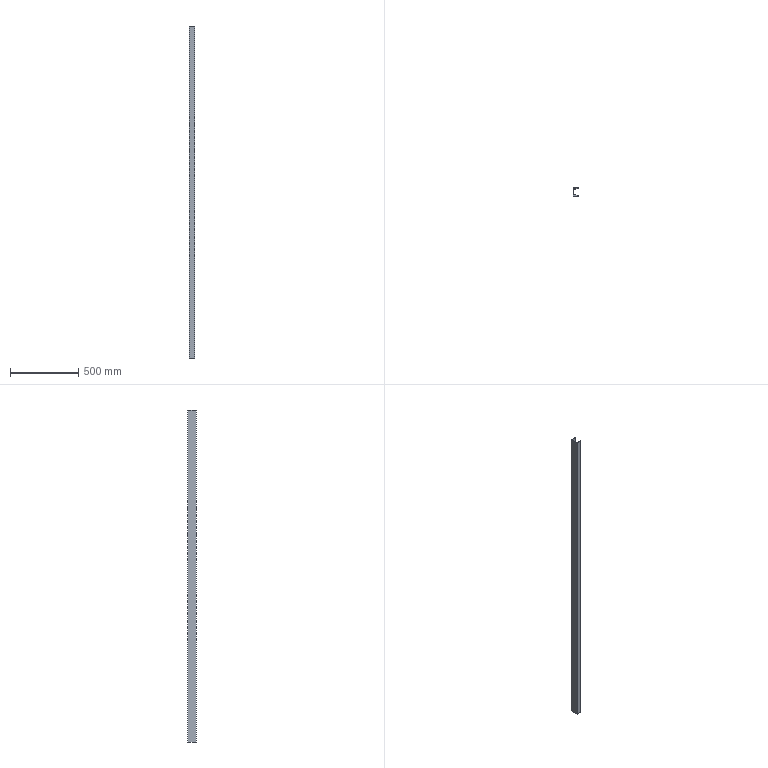Part | STEP file | 750038454 | 1 solid | 14 faces | box 40 x 63 x 2434 mm | volume 2055677 mm3 | plane 10 | cylinder 4 | commonest cylinder face diameters 7.6 x2 15 x2
STEP:
#1=CARTESIAN_POINT('',(0.,0.,2434.));
#2=VERTEX_POINT('',#1);
#3=CARTESIAN_POINT('',(0.,0.,0.));
#4=VERTEX_POINT('',#3);
#5=CARTESIAN_POINT('',(0.,0.,2434.));
#6=DIRECTION('',(0.,0.,-1.));
#7=VECTOR('',#6,1000.);
#8=LINE('',#5,#7);
#9=EDGE_CURVE('',#2,#4,#8,.T.);
#10=ORIENTED_EDGE('',*,*,#9,.F.);
#11=CARTESIAN_POINT('',(0.,63.,2434.));
#12=VERTEX_POINT('',#11);
#13=CARTESIAN_POINT('',(0.,63.,2434.));
#14=DIRECTION('',(0.,-1.,0.));
#15=VECTOR('',#14,1000.);
#16=LINE('',#13,#15);
#17=EDGE_CURVE('',#12,#2,#16,.T.);
#18=ORIENTED_EDGE('',*,*,#17,.F.);
#19=CARTESIAN_POINT('',(0.,63.,0.));
#20=VERTEX_POINT('',#19);
#21=CARTESIAN_POINT('',(0.,63.,2434.));
#22=DIRECTION('',(0.,0.,1.));
#23=VECTOR('',#22,1000.);
#24=LINE('',#21,#23);
#25=EDGE_CURVE('',#20,#12,#24,.T.);
#26=ORIENTED_EDGE('',*,*,#25,.F.);
#27=CARTESIAN_POINT('',(0.,63.,0.));
#28=DIRECTION('',(0.,1.,0.));
#29=VECTOR('',#28,1000.);
#30=LINE('',#27,#29);
#31=EDGE_CURVE('',#4,#20,#30,.T.);
#32=ORIENTED_EDGE('',*,*,#31,.F.);
#33=EDGE_LOOP('',(#10,#18,#26,#32));
#34=FACE_OUTER_BOUND('',#33,.T.);
#35=CARTESIAN_POINT('',(0.,63.,2434.));
#36=DIRECTION('',(1.,0.,0.));
#37=DIRECTION('',(0.,0.,-1.));
#38=AXIS2_PLACEMENT_3D('',#35,#36,#37);
#39=PLANE('',#38);
#40=ADVANCED_FACE('',(#34),#39,.F.);
#41=CARTESIAN_POINT('',(40.,63.,0.));
#42=VERTEX_POINT('',#41);
#43=CARTESIAN_POINT('',(36.2,63.,0.));
#44=DIRECTION('',(-1.,0.,0.));
#45=VECTOR('',#44,1000.);
#46=LINE('',#43,#45);
#47=EDGE_CURVE('',#42,#20,#46,.T.);
#48=ORIENTED_EDGE('',*,*,#47,.F.);
#49=CARTESIAN_POINT('',(40.,60.699,0.));
#50=VERTEX_POINT('',#49);
#51=CARTESIAN_POINT('',(40.,2.301,0.));
#52=DIRECTION('',(0.,1.,0.));
#53=VECTOR('',#52,1000.);
#54=LINE('',#51,#53);
#55=EDGE_CURVE('',#50,#42,#54,.T.);
#56=ORIENTED_EDGE('',*,*,#55,.F.);
#57=CARTESIAN_POINT('',(36.578,56.918,0.));
#58=VERTEX_POINT('',#57);
#59=CARTESIAN_POINT('',(36.2,60.699,0.));
#60=DIRECTION('',(0.,0.,1.));
#61=DIRECTION('',(-1.,0.,0.));
#62=AXIS2_PLACEMENT_3D('',#59,#60,#61);
#63=CIRCLE('',#62,3.8);
#64=EDGE_CURVE('',#58,#50,#63,.T.);
#65=ORIENTED_EDGE('',*,*,#64,.F.);
#66=CARTESIAN_POINT('',(11.554,54.415,0.));
#67=VERTEX_POINT('',#66);
#68=CARTESIAN_POINT('',(11.554,54.415,0.));
#69=DIRECTION('',(0.995,0.0995,0.));
#70=VECTOR('',#69,1000.);
#71=LINE('',#68,#70);
#72=EDGE_CURVE('',#67,#58,#71,.T.);
#73=ORIENTED_EDGE('',*,*,#72,.F.);
#74=CARTESIAN_POINT('',(4.8,46.953,0.));
#75=VERTEX_POINT('',#74);
#76=CARTESIAN_POINT('',(12.3,46.953,0.));
#77=DIRECTION('',(0.,0.,-1.));
#78=DIRECTION('',(-1.,0.,0.));
#79=AXIS2_PLACEMENT_3D('',#76,#77,#78);
#80=CIRCLE('',#79,7.5);
#81=EDGE_CURVE('',#75,#67,#80,.T.);
#82=ORIENTED_EDGE('',*,*,#81,.F.);
#83=CARTESIAN_POINT('',(4.8,16.047,0.));
#84=VERTEX_POINT('',#83);
#85=CARTESIAN_POINT('',(4.8,2.301,0.));
#86=DIRECTION('',(0.,1.,0.));
#87=VECTOR('',#86,1000.);
#88=LINE('',#85,#87);
#89=EDGE_CURVE('',#84,#75,#88,.T.);
#90=ORIENTED_EDGE('',*,*,#89,.F.);
#91=CARTESIAN_POINT('',(11.554,8.585,0.));
#92=VERTEX_POINT('',#91);
#93=CARTESIAN_POINT('',(12.3,16.047,0.));
#94=DIRECTION('',(0.,0.,-1.));
#95=DIRECTION('',(-1.,0.,0.));
#96=AXIS2_PLACEMENT_3D('',#93,#94,#95);
#97=CIRCLE('',#96,7.5);
#98=EDGE_CURVE('',#92,#84,#97,.T.);
#99=ORIENTED_EDGE('',*,*,#98,.F.);
#100=CARTESIAN_POINT('',(36.578,6.082,0.));
#101=VERTEX_POINT('',#100);
#102=CARTESIAN_POINT('',(36.578,6.082,0.));
#103=DIRECTION('',(-0.995,0.0995,0.));
#104=VECTOR('',#103,1000.);
#105=LINE('',#102,#104);
#106=EDGE_CURVE('',#101,#92,#105,.T.);
#107=ORIENTED_EDGE('',*,*,#106,.F.);
#108=CARTESIAN_POINT('',(40.,2.301,0.));
#109=VERTEX_POINT('',#108);
#110=CARTESIAN_POINT('',(36.2,2.301,0.));
#111=DIRECTION('',(0.,0.,1.));
#112=DIRECTION('',(-1.,0.,0.));
#113=AXIS2_PLACEMENT_3D('',#110,#111,#112);
#114=CIRCLE('',#113,3.8);
#115=EDGE_CURVE('',#109,#101,#114,.T.);
#116=ORIENTED_EDGE('',*,*,#115,.F.);
#117=CARTESIAN_POINT('',(40.,0.,0.));
#118=VERTEX_POINT('',#117);
#119=CARTESIAN_POINT('',(40.,2.301,0.));
#120=DIRECTION('',(0.,1.,0.));
#121=VECTOR('',#120,1000.);
#122=LINE('',#119,#121);
#123=EDGE_CURVE('',#118,#109,#122,.T.);
#124=ORIENTED_EDGE('',*,*,#123,.F.);
#125=CARTESIAN_POINT('',(36.2,0.,0.));
#126=DIRECTION('',(1.,0.,0.));
#127=VECTOR('',#126,1000.);
#128=LINE('',#125,#127);
#129=EDGE_CURVE('',#4,#118,#128,.T.);
#130=ORIENTED_EDGE('',*,*,#129,.F.);
#131=ORIENTED_EDGE('',*,*,#31,.T.);
#132=EDGE_LOOP('',(#48,#56,#65,#73,#82,#90,#99,#107,#116,#124,#130,#131));
#133=FACE_OUTER_BOUND('',#132,.T.);
#134=CARTESIAN_POINT('',(36.2,2.301,0.));
#135=DIRECTION('',(0.,0.,1.));
#136=DIRECTION('',(1.,0.,0.));
#137=AXIS2_PLACEMENT_3D('',#134,#135,#136);
#138=PLANE('',#137);
#139=ADVANCED_FACE('',(#133),#138,.F.);
#140=CARTESIAN_POINT('',(40.,0.,2434.));
#141=VERTEX_POINT('',#140);
#142=CARTESIAN_POINT('',(40.,0.,2434.));
#143=DIRECTION('',(0.,0.,-1.));
#144=VECTOR('',#143,1000.);
#145=LINE('',#142,#144);
#146=EDGE_CURVE('',#141,#118,#145,.T.);
#147=ORIENTED_EDGE('',*,*,#146,.F.);
#148=CARTESIAN_POINT('',(0.,0.,2434.));
#149=DIRECTION('',(1.,0.,0.));
#150=VECTOR('',#149,1000.);
#151=LINE('',#148,#150);
#152=EDGE_CURVE('',#2,#141,#151,.T.);
#153=ORIENTED_EDGE('',*,*,#152,.F.);
#154=ORIENTED_EDGE('',*,*,#9,.T.);
#155=ORIENTED_EDGE('',*,*,#129,.T.);
#156=EDGE_LOOP('',(#147,#153,#154,#155));
#157=FACE_OUTER_BOUND('',#156,.T.);
#158=CARTESIAN_POINT('',(0.,0.,2434.));
#159=DIRECTION('',(0.,1.,0.));
#160=DIRECTION('',(0.,0.,1.));
#161=AXIS2_PLACEMENT_3D('',#158,#159,#160);
#162=PLANE('',#161);
#163=ADVANCED_FACE('',(#157),#162,.F.);
#164=CARTESIAN_POINT('',(40.,60.699,2434.));
#165=VERTEX_POINT('',#164);
#166=CARTESIAN_POINT('',(40.,63.,2434.));
#167=VERTEX_POINT('',#166);
#168=CARTESIAN_POINT('',(40.,2.301,2434.));
#169=DIRECTION('',(0.,1.,0.));
#170=VECTOR('',#169,1000.);
#171=LINE('',#168,#170);
#172=EDGE_CURVE('',#165,#167,#171,.T.);
#173=ORIENTED_EDGE('',*,*,#172,.T.);
#174=CARTESIAN_POINT('',(36.2,63.,2434.));
#175=DIRECTION('',(-1.,0.,0.));
#176=VECTOR('',#175,1000.);
#177=LINE('',#174,#176);
#178=EDGE_CURVE('',#167,#12,#177,.T.);
#179=ORIENTED_EDGE('',*,*,#178,.T.);
#180=ORIENTED_EDGE('',*,*,#17,.T.);
#181=ORIENTED_EDGE('',*,*,#152,.T.);
#182=CARTESIAN_POINT('',(40.,2.301,2434.));
#183=VERTEX_POINT('',#182);
#184=CARTESIAN_POINT('',(40.,2.301,2434.));
#185=DIRECTION('',(0.,1.,0.));
#186=VECTOR('',#185,1000.);
#187=LINE('',#184,#186);
#188=EDGE_CURVE('',#141,#183,#187,.T.);
#189=ORIENTED_EDGE('',*,*,#188,.T.);
#190=CARTESIAN_POINT('',(36.578,6.082,2434.));
#191=VERTEX_POINT('',#190);
#192=CARTESIAN_POINT('',(36.2,2.301,2434.));
#193=DIRECTION('',(0.,0.,1.));
#194=DIRECTION('',(-1.,0.,0.));
#195=AXIS2_PLACEMENT_3D('',#192,#193,#194);
#196=CIRCLE('',#195,3.8);
#197=EDGE_CURVE('',#183,#191,#196,.T.);
#198=ORIENTED_EDGE('',*,*,#197,.T.);
#199=CARTESIAN_POINT('',(11.554,8.585,2434.));
#200=VERTEX_POINT('',#199);
#201=CARTESIAN_POINT('',(36.578,6.082,2434.));
#202=DIRECTION('',(-0.995,0.0995,0.));
#203=VECTOR('',#202,1000.);
#204=LINE('',#201,#203);
#205=EDGE_CURVE('',#191,#200,#204,.T.);
#206=ORIENTED_EDGE('',*,*,#205,.T.);
#207=CARTESIAN_POINT('',(4.8,16.047,2434.));
#208=VERTEX_POINT('',#207);
#209=CARTESIAN_POINT('',(12.3,16.047,2434.));
#210=DIRECTION('',(0.,0.,-1.));
#211=DIRECTION('',(-1.,0.,0.));
#212=AXIS2_PLACEMENT_3D('',#209,#210,#211);
#213=CIRCLE('',#212,7.5);
#214=EDGE_CURVE('',#200,#208,#213,.T.);
#215=ORIENTED_EDGE('',*,*,#214,.T.);
#216=CARTESIAN_POINT('',(4.8,46.953,2434.));
#217=VERTEX_POINT('',#216);
#218=CARTESIAN_POINT('',(4.8,2.301,2434.));
#219=DIRECTION('',(0.,1.,0.));
#220=VECTOR('',#219,1000.);
#221=LINE('',#218,#220);
#222=EDGE_CURVE('',#208,#217,#221,.T.);
#223=ORIENTED_EDGE('',*,*,#222,.T.);
#224=CARTESIAN_POINT('',(11.554,54.415,2434.));
#225=VERTEX_POINT('',#224);
#226=CARTESIAN_POINT('',(12.3,46.953,2434.));
#227=DIRECTION('',(0.,0.,-1.));
#228=DIRECTION('',(-1.,0.,0.));
#229=AXIS2_PLACEMENT_3D('',#226,#227,#228);
#230=CIRCLE('',#229,7.5);
#231=EDGE_CURVE('',#217,#225,#230,.T.);
#232=ORIENTED_EDGE('',*,*,#231,.T.);
#233=CARTESIAN_POINT('',(36.578,56.918,2434.));
#234=VERTEX_POINT('',#233);
#235=CARTESIAN_POINT('',(11.554,54.415,2434.));
#236=DIRECTION('',(0.995,0.0995,0.));
#237=VECTOR('',#236,1000.);
#238=LINE('',#235,#237);
#239=EDGE_CURVE('',#225,#234,#238,.T.);
#240=ORIENTED_EDGE('',*,*,#239,.T.);
#241=CARTESIAN_POINT('',(36.2,60.699,2434.));
#242=DIRECTION('',(0.,0.,1.));
#243=DIRECTION('',(-1.,0.,0.));
#244=AXIS2_PLACEMENT_3D('',#241,#242,#243);
#245=CIRCLE('',#244,3.8);
#246=EDGE_CURVE('',#234,#165,#245,.T.);
#247=ORIENTED_EDGE('',*,*,#246,.T.);
#248=EDGE_LOOP('',(#173,#179,#180,#181,#189,#198,#206,#215,#223,#232,#240,#247));
#249=FACE_OUTER_BOUND('',#248,.T.);
#250=CARTESIAN_POINT('',(36.2,2.301,2434.));
#251=DIRECTION('',(0.,0.,1.));
#252=DIRECTION('',(1.,0.,0.));
#253=AXIS2_PLACEMENT_3D('',#250,#251,#252);
#254=PLANE('',#253);
#255=ADVANCED_FACE('',(#249),#254,.T.);
#256=ORIENTED_EDGE('',*,*,#25,.T.);
#257=ORIENTED_EDGE('',*,*,#178,.F.);
#258=CARTESIAN_POINT('',(40.,63.,2434.));
#259=DIRECTION('',(0.,0.,1.));
#260=VECTOR('',#259,1000.);
#261=LINE('',#258,#260);
#262=EDGE_CURVE('',#42,#167,#261,.T.);
#263=ORIENTED_EDGE('',*,*,#262,.F.);
#264=ORIENTED_EDGE('',*,*,#47,.T.);
#265=EDGE_LOOP('',(#256,#257,#263,#264));
#266=FACE_OUTER_BOUND('',#265,.T.);
#267=CARTESIAN_POINT('',(40.,63.,2434.));
#268=DIRECTION('',(0.,-1.,0.));
#269=DIRECTION('',(0.,0.,-1.));
#270=AXIS2_PLACEMENT_3D('',#267,#268,#269);
#271=PLANE('',#270);
#272=ADVANCED_FACE('',(#266),#271,.F.);
#273=ORIENTED_EDGE('',*,*,#262,.T.);
#274=ORIENTED_EDGE('',*,*,#172,.F.);
#275=CARTESIAN_POINT('',(40.,60.699,2434.));
#276=DIRECTION('',(0.,0.,1.));
#277=VECTOR('',#276,1000.);
#278=LINE('',#275,#277);
#279=EDGE_CURVE('',#50,#165,#278,.T.);
#280=ORIENTED_EDGE('',*,*,#279,.F.);
#281=ORIENTED_EDGE('',*,*,#55,.T.);
#282=EDGE_LOOP('',(#273,#274,#280,#281));
#283=FACE_OUTER_BOUND('',#282,.T.);
#284=CARTESIAN_POINT('',(40.,60.699,2434.));
#285=DIRECTION('',(-1.,0.,0.));
#286=DIRECTION('',(0.,-1.,0.));
#287=AXIS2_PLACEMENT_3D('',#284,#285,#286);
#288=PLANE('',#287);
#289=ADVANCED_FACE('',(#283),#288,.F.);
#290=ORIENTED_EDGE('',*,*,#246,.F.);
#291=CARTESIAN_POINT('',(36.578,56.918,2434.));
#292=DIRECTION('',(0.,0.,-1.));
#293=VECTOR('',#292,1000.);
#294=LINE('',#291,#293);
#295=EDGE_CURVE('',#234,#58,#294,.T.);
#296=ORIENTED_EDGE('',*,*,#295,.T.);
#297=ORIENTED_EDGE('',*,*,#64,.T.);
#298=ORIENTED_EDGE('',*,*,#279,.T.);
#299=EDGE_LOOP('',(#290,#296,#297,#298));
#300=FACE_OUTER_BOUND('',#299,.T.);
#301=CARTESIAN_POINT('',(36.2,60.699,2434.));
#302=DIRECTION('',(0.,0.,-1.));
#303=DIRECTION('',(-1.,0.,0.));
#304=AXIS2_PLACEMENT_3D('',#301,#302,#303);
#305=CYLINDRICAL_SURFACE('',#304,3.8);
#306=ADVANCED_FACE('',(#300),#305,.T.);
#307=ORIENTED_EDGE('',*,*,#295,.F.);
#308=ORIENTED_EDGE('',*,*,#239,.F.);
#309=CARTESIAN_POINT('',(11.554,54.415,2434.));
#310=DIRECTION('',(0.,0.,1.));
#311=VECTOR('',#310,1000.);
#312=LINE('',#309,#311);
#313=EDGE_CURVE('',#67,#225,#312,.T.);
#314=ORIENTED_EDGE('',*,*,#313,.F.);
#315=ORIENTED_EDGE('',*,*,#72,.T.);
#316=EDGE_LOOP('',(#307,#308,#314,#315));
#317=FACE_OUTER_BOUND('',#316,.T.);
#318=CARTESIAN_POINT('',(11.554,54.415,2434.));
#319=DIRECTION('',(-0.0995,0.995,0.));
#320=DIRECTION('',(-0.995,-0.0995,0.));
#321=AXIS2_PLACEMENT_3D('',#318,#319,#320);
#322=PLANE('',#321);
#323=ADVANCED_FACE('',(#317),#322,.F.);
#324=ORIENTED_EDGE('',*,*,#313,.T.);
#325=ORIENTED_EDGE('',*,*,#231,.F.);
#326=CARTESIAN_POINT('',(4.8,46.953,2434.));
#327=DIRECTION('',(0.,0.,1.));
#328=VECTOR('',#327,1000.);
#329=LINE('',#326,#328);
#330=EDGE_CURVE('',#75,#217,#329,.T.);
#331=ORIENTED_EDGE('',*,*,#330,.F.);
#332=ORIENTED_EDGE('',*,*,#81,.T.);
#333=EDGE_LOOP('',(#324,#325,#331,#332));
#334=FACE_OUTER_BOUND('',#333,.T.);
#335=CARTESIAN_POINT('',(12.3,46.953,2434.));
#336=DIRECTION('',(0.,0.,-1.));
#337=DIRECTION('',(-1.,0.,0.));
#338=AXIS2_PLACEMENT_3D('',#335,#336,#337);
#339=CYLINDRICAL_SURFACE('',#338,7.5);
#340=ADVANCED_FACE('',(#334),#339,.F.);
#341=ORIENTED_EDGE('',*,*,#330,.T.);
#342=ORIENTED_EDGE('',*,*,#222,.F.);
#343=CARTESIAN_POINT('',(4.8,16.047,2434.));
#344=DIRECTION('',(0.,0.,1.));
#345=VECTOR('',#344,1000.);
#346=LINE('',#343,#345);
#347=EDGE_CURVE('',#84,#208,#346,.T.);
#348=ORIENTED_EDGE('',*,*,#347,.F.);
#349=ORIENTED_EDGE('',*,*,#89,.T.);
#350=EDGE_LOOP('',(#341,#342,#348,#349));
#351=FACE_OUTER_BOUND('',#350,.T.);
#352=CARTESIAN_POINT('',(4.8,16.047,2434.));
#353=DIRECTION('',(-1.,0.,0.));
#354=DIRECTION('',(0.,-1.,0.));
#355=AXIS2_PLACEMENT_3D('',#352,#353,#354);
#356=PLANE('',#355);
#357=ADVANCED_FACE('',(#351),#356,.F.);
#358=ORIENTED_EDGE('',*,*,#347,.T.);
#359=ORIENTED_EDGE('',*,*,#214,.F.);
#360=CARTESIAN_POINT('',(11.554,8.585,2434.));
#361=DIRECTION('',(0.,0.,1.));
#362=VECTOR('',#361,1000.);
#363=LINE('',#360,#362);
#364=EDGE_CURVE('',#92,#200,#363,.T.);
#365=ORIENTED_EDGE('',*,*,#364,.F.);
#366=ORIENTED_EDGE('',*,*,#98,.T.);
#367=EDGE_LOOP('',(#358,#359,#365,#366));
#368=FACE_OUTER_BOUND('',#367,.T.);
#369=CARTESIAN_POINT('',(12.3,16.047,2434.));
#370=DIRECTION('',(0.,0.,-1.));
#371=DIRECTION('',(-1.,0.,0.));
#372=AXIS2_PLACEMENT_3D('',#369,#370,#371);
#373=CYLINDRICAL_SURFACE('',#372,7.5);
#374=ADVANCED_FACE('',(#368),#373,.F.);
#375=ORIENTED_EDGE('',*,*,#364,.T.);
#376=ORIENTED_EDGE('',*,*,#205,.F.);
#377=CARTESIAN_POINT('',(36.578,6.082,2434.));
#378=DIRECTION('',(0.,0.,1.));
#379=VECTOR('',#378,1000.);
#380=LINE('',#377,#379);
#381=EDGE_CURVE('',#101,#191,#380,.T.);
#382=ORIENTED_EDGE('',*,*,#381,.F.);
#383=ORIENTED_EDGE('',*,*,#106,.T.);
#384=EDGE_LOOP('',(#375,#376,#382,#383));
#385=FACE_OUTER_BOUND('',#384,.T.);
#386=CARTESIAN_POINT('',(36.578,6.082,2434.));
#387=DIRECTION('',(-0.0995,-0.995,0.));
#388=DIRECTION('',(0.995,-0.0995,0.));
#389=AXIS2_PLACEMENT_3D('',#386,#387,#388);
#390=PLANE('',#389);
#391=ADVANCED_FACE('',(#385),#390,.F.);
#392=ORIENTED_EDGE('',*,*,#197,.F.);
#393=CARTESIAN_POINT('',(40.,2.301,2434.));
#394=DIRECTION('',(0.,0.,-1.));
#395=VECTOR('',#394,1000.);
#396=LINE('',#393,#395);
#397=EDGE_CURVE('',#183,#109,#396,.T.);
#398=ORIENTED_EDGE('',*,*,#397,.T.);
#399=ORIENTED_EDGE('',*,*,#115,.T.);
#400=ORIENTED_EDGE('',*,*,#381,.T.);
#401=EDGE_LOOP('',(#392,#398,#399,#400));
#402=FACE_OUTER_BOUND('',#401,.T.);
#403=CARTESIAN_POINT('',(36.2,2.301,2434.));
#404=DIRECTION('',(0.,0.,-1.));
#405=DIRECTION('',(-1.,0.,0.));
#406=AXIS2_PLACEMENT_3D('',#403,#404,#405);
#407=CYLINDRICAL_SURFACE('',#406,3.8);
#408=ADVANCED_FACE('',(#402),#407,.T.);
#409=ORIENTED_EDGE('',*,*,#397,.F.);
#410=ORIENTED_EDGE('',*,*,#188,.F.);
#411=ORIENTED_EDGE('',*,*,#146,.T.);
#412=ORIENTED_EDGE('',*,*,#123,.T.);
#413=EDGE_LOOP('',(#409,#410,#411,#412));
#414=FACE_OUTER_BOUND('',#413,.T.);
#415=CARTESIAN_POINT('',(40.,0.,2434.));
#416=DIRECTION('',(-1.,0.,0.));
#417=DIRECTION('',(0.,0.,1.));
#418=AXIS2_PLACEMENT_3D('',#415,#416,#417);
#419=PLANE('',#418);
#420=ADVANCED_FACE('',(#414),#419,.F.);
#421=CLOSED_SHELL('',(#40,#139,#163,#255,#272,#289,#306,#323,#340,#357,#374,#391,#408,#420));
#422=MANIFOLD_SOLID_BREP('',#421);
#423=CARTESIAN_POINT('',(0.,0.,0.));
#424=DIRECTION('',(0.,0.,1.));
#425=DIRECTION('',(1.,0.,0.));
#426=AXIS2_PLACEMENT_3D('',#423,#424,#425);
#427=(LENGTH_UNIT()NAMED_UNIT(*)SI_UNIT(.MILLI.,.METRE.));
#428=UNCERTAINTY_MEASURE_WITH_UNIT(LENGTH_MEASURE(0.00001),#427,'','');
#429=(NAMED_UNIT(*)PLANE_ANGLE_UNIT()SI_UNIT($,.RADIAN.));
#430=(NAMED_UNIT(*)SI_UNIT($,.STERADIAN.)SOLID_ANGLE_UNIT());
#431=(GEOMETRIC_REPRESENTATION_CONTEXT(3)GLOBAL_UNCERTAINTY_ASSIGNED_CONTEXT((#428))GLOBAL_UNIT_ASSIGNED_CONTEXT((#427,#429,#430))REPRESENTATION_CONTEXT('',''));
#432=ADVANCED_BREP_SHAPE_REPRESENTATION('',(#422,#426),#431);